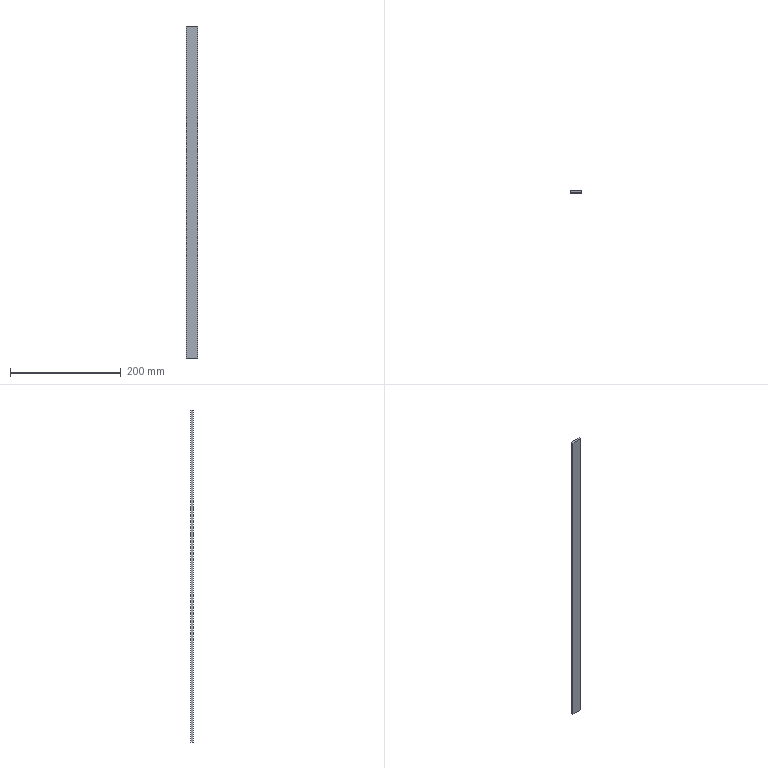Part | STEP file | Guide wheel mechanism revised.sldasm-Part-86 | 1 solid | 6 faces | box 20 x 4.19 x 600 mm | volume 50281 mm3 | plane 6
STEP:
#1=CARTESIAN_POINT('',(130.988,-28.55,-600.));
#2=VERTEX_POINT('',#1);
#3=CARTESIAN_POINT('',(130.988,-24.36,-600.));
#4=VERTEX_POINT('',#3);
#5=CARTESIAN_POINT('',(130.988,-24.36,-600.));
#6=DIRECTION('',(0.,1.,0.));
#7=VECTOR('',#6,1000.);
#8=LINE('',#5,#7);
#9=EDGE_CURVE('',#2,#4,#8,.T.);
#10=ORIENTED_EDGE('',*,*,#9,.F.);
#11=CARTESIAN_POINT('',(130.988,-28.55,0.));
#12=VERTEX_POINT('',#11);
#13=CARTESIAN_POINT('',(130.988,-28.55,-620.57));
#14=DIRECTION('',(0.,0.,1.));
#15=VECTOR('',#14,1000.);
#16=LINE('',#13,#15);
#17=EDGE_CURVE('',#2,#12,#16,.T.);
#18=ORIENTED_EDGE('',*,*,#17,.T.);
#19=CARTESIAN_POINT('',(130.988,-24.36,0.));
#20=VERTEX_POINT('',#19);
#21=CARTESIAN_POINT('',(130.988,-24.36,0.));
#22=DIRECTION('',(0.,-1.,0.));
#23=VECTOR('',#22,1000.);
#24=LINE('',#21,#23);
#25=EDGE_CURVE('',#20,#12,#24,.T.);
#26=ORIENTED_EDGE('',*,*,#25,.F.);
#27=CARTESIAN_POINT('',(130.988,-24.36,-620.57));
#28=DIRECTION('',(0.,0.,1.));
#29=VECTOR('',#28,1000.);
#30=LINE('',#27,#29);
#31=EDGE_CURVE('',#4,#20,#30,.T.);
#32=ORIENTED_EDGE('',*,*,#31,.F.);
#33=EDGE_LOOP('',(#10,#18,#26,#32));
#34=FACE_OUTER_BOUND('',#33,.T.);
#35=CARTESIAN_POINT('',(130.988,-24.36,-620.57));
#36=DIRECTION('',(-1.,0.,0.));
#37=DIRECTION('',(0.,0.,1.));
#38=AXIS2_PLACEMENT_3D('',#35,#36,#37);
#39=PLANE('',#38);
#40=ADVANCED_FACE('',(#34),#39,.T.);
#41=CARTESIAN_POINT('',(150.988,-24.36,-600.));
#42=VERTEX_POINT('',#41);
#43=CARTESIAN_POINT('',(130.988,-24.36,-600.));
#44=DIRECTION('',(1.,0.,0.));
#45=VECTOR('',#44,1000.);
#46=LINE('',#43,#45);
#47=EDGE_CURVE('',#4,#42,#46,.T.);
#48=ORIENTED_EDGE('',*,*,#47,.F.);
#49=ORIENTED_EDGE('',*,*,#31,.T.);
#50=CARTESIAN_POINT('',(150.988,-24.36,0.));
#51=VERTEX_POINT('',#50);
#52=CARTESIAN_POINT('',(130.988,-24.36,0.));
#53=DIRECTION('',(-1.,0.,0.));
#54=VECTOR('',#53,1000.);
#55=LINE('',#52,#54);
#56=EDGE_CURVE('',#51,#20,#55,.T.);
#57=ORIENTED_EDGE('',*,*,#56,.F.);
#58=CARTESIAN_POINT('',(150.988,-24.36,-620.57));
#59=DIRECTION('',(0.,0.,1.));
#60=VECTOR('',#59,1000.);
#61=LINE('',#58,#60);
#62=EDGE_CURVE('',#42,#51,#61,.T.);
#63=ORIENTED_EDGE('',*,*,#62,.F.);
#64=EDGE_LOOP('',(#48,#49,#57,#63));
#65=FACE_OUTER_BOUND('',#64,.T.);
#66=CARTESIAN_POINT('',(130.988,-24.36,-620.57));
#67=DIRECTION('',(0.,1.,0.));
#68=DIRECTION('',(-1.,0.,0.));
#69=AXIS2_PLACEMENT_3D('',#66,#67,#68);
#70=PLANE('',#69);
#71=ADVANCED_FACE('',(#65),#70,.T.);
#72=CARTESIAN_POINT('',(150.988,-28.55,-600.));
#73=VERTEX_POINT('',#72);
#74=CARTESIAN_POINT('',(150.988,-24.36,-600.));
#75=DIRECTION('',(0.,-1.,0.));
#76=VECTOR('',#75,1000.);
#77=LINE('',#74,#76);
#78=EDGE_CURVE('',#42,#73,#77,.T.);
#79=ORIENTED_EDGE('',*,*,#78,.F.);
#80=ORIENTED_EDGE('',*,*,#62,.T.);
#81=CARTESIAN_POINT('',(150.988,-28.55,0.));
#82=VERTEX_POINT('',#81);
#83=CARTESIAN_POINT('',(150.988,-24.36,0.));
#84=DIRECTION('',(0.,1.,0.));
#85=VECTOR('',#84,1000.);
#86=LINE('',#83,#85);
#87=EDGE_CURVE('',#82,#51,#86,.T.);
#88=ORIENTED_EDGE('',*,*,#87,.F.);
#89=CARTESIAN_POINT('',(150.988,-28.55,-620.57));
#90=DIRECTION('',(0.,0.,1.));
#91=VECTOR('',#90,1000.);
#92=LINE('',#89,#91);
#93=EDGE_CURVE('',#73,#82,#92,.T.);
#94=ORIENTED_EDGE('',*,*,#93,.F.);
#95=EDGE_LOOP('',(#79,#80,#88,#94));
#96=FACE_OUTER_BOUND('',#95,.T.);
#97=CARTESIAN_POINT('',(150.988,-24.36,-620.57));
#98=DIRECTION('',(1.,0.,0.));
#99=DIRECTION('',(0.,0.,-1.));
#100=AXIS2_PLACEMENT_3D('',#97,#98,#99);
#101=PLANE('',#100);
#102=ADVANCED_FACE('',(#96),#101,.T.);
#103=CARTESIAN_POINT('',(130.988,-28.55,-600.));
#104=DIRECTION('',(-1.,0.,0.));
#105=VECTOR('',#104,1000.);
#106=LINE('',#103,#105);
#107=EDGE_CURVE('',#73,#2,#106,.T.);
#108=ORIENTED_EDGE('',*,*,#107,.F.);
#109=ORIENTED_EDGE('',*,*,#93,.T.);
#110=CARTESIAN_POINT('',(130.988,-28.55,0.));
#111=DIRECTION('',(1.,0.,0.));
#112=VECTOR('',#111,1000.);
#113=LINE('',#110,#112);
#114=EDGE_CURVE('',#12,#82,#113,.T.);
#115=ORIENTED_EDGE('',*,*,#114,.F.);
#116=ORIENTED_EDGE('',*,*,#17,.F.);
#117=EDGE_LOOP('',(#108,#109,#115,#116));
#118=FACE_OUTER_BOUND('',#117,.T.);
#119=CARTESIAN_POINT('',(130.988,-28.55,-620.57));
#120=DIRECTION('',(0.,-1.,0.));
#121=DIRECTION('',(1.,0.,0.));
#122=AXIS2_PLACEMENT_3D('',#119,#120,#121);
#123=PLANE('',#122);
#124=ADVANCED_FACE('',(#118),#123,.T.);
#125=ORIENTED_EDGE('',*,*,#25,.T.);
#126=ORIENTED_EDGE('',*,*,#114,.T.);
#127=ORIENTED_EDGE('',*,*,#87,.T.);
#128=ORIENTED_EDGE('',*,*,#56,.T.);
#129=EDGE_LOOP('',(#125,#126,#127,#128));
#130=FACE_OUTER_BOUND('',#129,.T.);
#131=CARTESIAN_POINT('',(0.,0.,0.));
#132=DIRECTION('',(0.,0.,1.));
#133=DIRECTION('',(1.,0.,0.));
#134=AXIS2_PLACEMENT_3D('',#131,#132,#133);
#135=PLANE('',#134);
#136=ADVANCED_FACE('',(#130),#135,.T.);
#137=ORIENTED_EDGE('',*,*,#9,.T.);
#138=ORIENTED_EDGE('',*,*,#47,.T.);
#139=ORIENTED_EDGE('',*,*,#78,.T.);
#140=ORIENTED_EDGE('',*,*,#107,.T.);
#141=EDGE_LOOP('',(#137,#138,#139,#140));
#142=FACE_OUTER_BOUND('',#141,.T.);
#143=CARTESIAN_POINT('',(-14.837,-23.55,-600.));
#144=DIRECTION('',(0.,0.,1.));
#145=DIRECTION('',(1.,0.,0.));
#146=AXIS2_PLACEMENT_3D('',#143,#144,#145);
#147=PLANE('',#146);
#148=ADVANCED_FACE('',(#142),#147,.F.);
#149=CLOSED_SHELL('',(#40,#71,#102,#124,#136,#148));
#150=MANIFOLD_SOLID_BREP('',#149);
#151=CARTESIAN_POINT('',(0.,0.,0.));
#152=DIRECTION('',(0.,0.,1.));
#153=DIRECTION('',(1.,0.,0.));
#154=AXIS2_PLACEMENT_3D('',#151,#152,#153);
#155=(LENGTH_UNIT()NAMED_UNIT(*)SI_UNIT(.MILLI.,.METRE.));
#156=UNCERTAINTY_MEASURE_WITH_UNIT(LENGTH_MEASURE(0.00001),#155,'','');
#157=(NAMED_UNIT(*)PLANE_ANGLE_UNIT()SI_UNIT($,.RADIAN.));
#158=(NAMED_UNIT(*)SI_UNIT($,.STERADIAN.)SOLID_ANGLE_UNIT());
#159=(GEOMETRIC_REPRESENTATION_CONTEXT(3)GLOBAL_UNCERTAINTY_ASSIGNED_CONTEXT((#156))GLOBAL_UNIT_ASSIGNED_CONTEXT((#155,#157,#158))REPRESENTATION_CONTEXT('',''));
#160=ADVANCED_BREP_SHAPE_REPRESENTATION('',(#150,#154),#159);